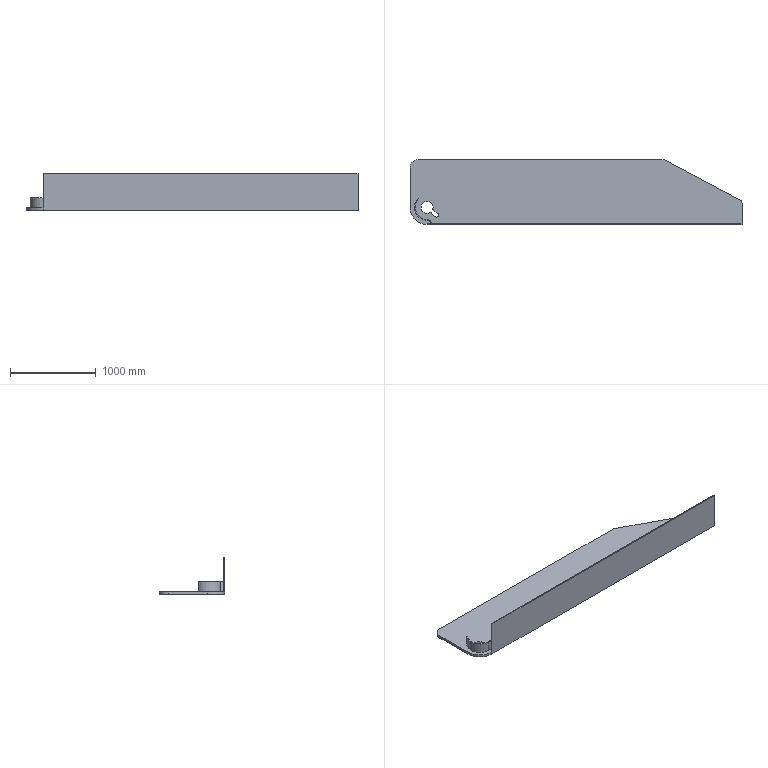Part | NX | features 顶梁侧护板右 2 | 1 solid | 26 faces | box 3880 x 760 x 430 mm | volume 99045232 mm3 | plane 14 | cylinder 12 | commonest cylinder face diameters 40 x2 50 x1 76 x1 96 x1 100 x1 140 x1
STEP:
#1=CARTESIAN_POINT('',(-1665.412,-207.572,-800.));
#2=VERTEX_POINT('',#1);
#3=CARTESIAN_POINT('',(-1673.791,-186.574,-800.));
#4=VERTEX_POINT('',#3);
#5=CARTESIAN_POINT('',(-1654.278,-190.958,-800.));
#6=DIRECTION('',(0.,0.,-1.));
#7=DIRECTION('',(1.,0.,0.));
#8=AXIS2_PLACEMENT_3D('',#5,#6,#7);
#9=CIRCLE('',#8,20.);
#10=EDGE_CURVE('',#2,#4,#9,.T.);
#11=ORIENTED_EDGE('',*,*,#10,.F.);
#12=CARTESIAN_POINT('',(-1619.198,-238.543,-800.));
#13=VERTEX_POINT('',#12);
#14=CARTESIAN_POINT('',(-1619.198,-238.543,-800.));
#15=DIRECTION('',(-0.8307,0.5567,0.));
#16=VECTOR('',#15,1000.);
#17=LINE('',#14,#16);
#18=EDGE_CURVE('',#13,#2,#17,.T.);
#19=ORIENTED_EDGE('',*,*,#18,.F.);
#20=CARTESIAN_POINT('',(-1650.504,-277.274,-800.));
#21=VERTEX_POINT('',#20);
#22=CARTESIAN_POINT('',(-1633.116,-259.311,-800.));
#23=DIRECTION('',(0.,0.,1.));
#24=DIRECTION('',(1.,0.,0.));
#25=AXIS2_PLACEMENT_3D('',#22,#23,#24);
#26=CIRCLE('',#25,25.);
#27=EDGE_CURVE('',#21,#13,#26,.T.);
#28=ORIENTED_EDGE('',*,*,#27,.F.);
#29=CARTESIAN_POINT('',(-1690.478,-238.583,-800.));
#30=VERTEX_POINT('',#29);
#31=CARTESIAN_POINT('',(-1690.478,-238.583,-800.));
#32=DIRECTION('',(0.7185,-0.6955,0.));
#33=VECTOR('',#32,1000.);
#34=LINE('',#31,#33);
#35=EDGE_CURVE('',#30,#21,#34,.T.);
#36=ORIENTED_EDGE('',*,*,#35,.F.);
#37=CARTESIAN_POINT('',(-1712.765,-234.793,-800.));
#38=VERTEX_POINT('',#37);
#39=CARTESIAN_POINT('',(-1704.387,-252.954,-800.));
#40=DIRECTION('',(0.,0.,-1.));
#41=DIRECTION('',(1.,0.,0.));
#42=AXIS2_PLACEMENT_3D('',#39,#40,#41);
#43=CIRCLE('',#42,20.);
#44=EDGE_CURVE('',#38,#30,#43,.T.);
#45=ORIENTED_EDGE('',*,*,#44,.F.);
#46=CARTESIAN_POINT('',(-1742.089,-171.231,-800.));
#47=DIRECTION('',(0.,0.,1.));
#48=DIRECTION('',(1.,0.,0.));
#49=AXIS2_PLACEMENT_3D('',#46,#47,#48);
#50=CIRCLE('',#49,70.);
#51=EDGE_CURVE('',#4,#38,#50,.T.);
#52=ORIENTED_EDGE('',*,*,#51,.F.);
#53=EDGE_LOOP('',(#11,#19,#28,#36,#45,#52));
#54=FACE_BOUND('',#53,.T.);
#55=CARTESIAN_POINT('',(-1742.089,-311.231,-800.));
#56=VERTEX_POINT('',#55);
#57=CARTESIAN_POINT('',(-1694.089,-359.231,-800.));
#58=VERTEX_POINT('',#57);
#59=CARTESIAN_POINT('',(-1742.089,-359.231,-800.));
#60=DIRECTION('',(0.,0.,-1.));
#61=DIRECTION('',(-1.,0.,0.));
#62=AXIS2_PLACEMENT_3D('',#59,#60,#61);
#63=CIRCLE('',#62,48.);
#64=EDGE_CURVE('',#56,#58,#63,.T.);
#65=ORIENTED_EDGE('',*,*,#64,.T.);
#66=CARTESIAN_POINT('',(1937.911,-359.231,-800.));
#67=VERTEX_POINT('',#66);
#68=CARTESIAN_POINT('',(1937.911,-359.231,-800.));
#69=DIRECTION('',(1.,0.,0.));
#70=VECTOR('',#69,1000.);
#71=LINE('',#68,#70);
#72=EDGE_CURVE('',#58,#67,#71,.T.);
#73=ORIENTED_EDGE('',*,*,#72,.T.);
#74=CARTESIAN_POINT('',(1937.911,-126.493,-800.));
#75=VERTEX_POINT('',#74);
#76=CARTESIAN_POINT('',(1937.911,-371.231,-800.));
#77=DIRECTION('',(0.,1.,0.));
#78=VECTOR('',#77,1000.);
#79=LINE('',#76,#78);
#80=EDGE_CURVE('',#67,#75,#79,.T.);
#81=ORIENTED_EDGE('',*,*,#80,.T.);
#82=CARTESIAN_POINT('',(1911.333,-82.318,-800.));
#83=VERTEX_POINT('',#82);
#84=CARTESIAN_POINT('',(1887.911,-126.493,-800.));
#85=DIRECTION('',(0.,0.,1.));
#86=DIRECTION('',(1.,0.,0.));
#87=AXIS2_PLACEMENT_3D('',#84,#85,#86);
#88=CIRCLE('',#87,50.);
#89=EDGE_CURVE('',#75,#83,#88,.T.);
#90=ORIENTED_EDGE('',*,*,#89,.T.);
#91=CARTESIAN_POINT('',(1040.435,379.448,-800.));
#92=VERTEX_POINT('',#91);
#93=CARTESIAN_POINT('',(1911.333,-82.318,-800.));
#94=DIRECTION('',(-0.8835,0.4684,0.));
#95=VECTOR('',#94,1000.);
#96=LINE('',#93,#95);
#97=EDGE_CURVE('',#83,#92,#96,.T.);
#98=ORIENTED_EDGE('',*,*,#97,.T.);
#99=CARTESIAN_POINT('',(1002.96,388.769,-800.));
#100=VERTEX_POINT('',#99);
#101=CARTESIAN_POINT('',(1002.96,308.769,-800.));
#102=DIRECTION('',(0.,0.,1.));
#103=DIRECTION('',(1.,0.,0.));
#104=AXIS2_PLACEMENT_3D('',#101,#102,#103);
#105=CIRCLE('',#104,80.);
#106=EDGE_CURVE('',#92,#100,#105,.T.);
#107=ORIENTED_EDGE('',*,*,#106,.T.);
#108=CARTESIAN_POINT('',(-1842.089,388.769,-800.));
#109=VERTEX_POINT('',#108);
#110=CARTESIAN_POINT('',(1002.96,388.769,-800.));
#111=DIRECTION('',(-1.,0.,0.));
#112=VECTOR('',#111,1000.);
#113=LINE('',#110,#112);
#114=EDGE_CURVE('',#100,#109,#113,.T.);
#115=ORIENTED_EDGE('',*,*,#114,.T.);
#116=CARTESIAN_POINT('',(-1942.089,288.769,-800.));
#117=VERTEX_POINT('',#116);
#118=CARTESIAN_POINT('',(-1842.089,288.769,-800.));
#119=DIRECTION('',(0.,0.,1.));
#120=DIRECTION('',(1.,0.,0.));
#121=AXIS2_PLACEMENT_3D('',#118,#119,#120);
#122=CIRCLE('',#121,100.);
#123=EDGE_CURVE('',#109,#117,#122,.T.);
#124=ORIENTED_EDGE('',*,*,#123,.T.);
#125=CARTESIAN_POINT('',(-1942.089,-171.231,-800.));
#126=VERTEX_POINT('',#125);
#127=CARTESIAN_POINT('',(-1942.089,288.769,-800.));
#128=DIRECTION('',(0.,-1.,0.));
#129=VECTOR('',#128,1000.);
#130=LINE('',#127,#129);
#131=EDGE_CURVE('',#117,#126,#130,.T.);
#132=ORIENTED_EDGE('',*,*,#131,.T.);
#133=CARTESIAN_POINT('',(-1742.089,-371.231,-800.));
#134=VERTEX_POINT('',#133);
#135=CARTESIAN_POINT('',(-1742.089,-171.231,-800.));
#136=DIRECTION('',(0.,0.,1.));
#137=DIRECTION('',(1.,0.,0.));
#138=AXIS2_PLACEMENT_3D('',#135,#136,#137);
#139=CIRCLE('',#138,200.);
#140=EDGE_CURVE('',#126,#134,#139,.T.);
#141=ORIENTED_EDGE('',*,*,#140,.T.);
#142=CARTESIAN_POINT('',(-1742.089,-359.231,-800.));
#143=VERTEX_POINT('',#142);
#144=CARTESIAN_POINT('',(-1742.089,-371.231,-800.));
#145=DIRECTION('',(0.,1.,0.));
#146=VECTOR('',#145,1000.);
#147=LINE('',#144,#146);
#148=EDGE_CURVE('',#134,#143,#147,.T.);
#149=ORIENTED_EDGE('',*,*,#148,.T.);
#150=CARTESIAN_POINT('',(-1704.089,-359.231,-800.));
#151=VERTEX_POINT('',#150);
#152=CARTESIAN_POINT('',(1937.911,-359.231,-800.));
#153=DIRECTION('',(1.,0.,0.));
#154=VECTOR('',#153,1000.);
#155=LINE('',#152,#154);
#156=EDGE_CURVE('',#143,#151,#155,.T.);
#157=ORIENTED_EDGE('',*,*,#156,.T.);
#158=CARTESIAN_POINT('',(-1742.089,-321.231,-800.));
#159=VERTEX_POINT('',#158);
#160=CARTESIAN_POINT('',(-1742.089,-359.231,-800.));
#161=DIRECTION('',(0.,0.,1.));
#162=DIRECTION('',(-1.,0.,0.));
#163=AXIS2_PLACEMENT_3D('',#160,#161,#162);
#164=CIRCLE('',#163,38.);
#165=EDGE_CURVE('',#151,#159,#164,.T.);
#166=ORIENTED_EDGE('',*,*,#165,.T.);
#167=CARTESIAN_POINT('',(-1848.155,-65.165,-800.));
#168=VERTEX_POINT('',#167);
#169=CARTESIAN_POINT('',(-1742.089,-171.231,-800.));
#170=DIRECTION('',(0.,0.,-1.));
#171=DIRECTION('',(-1.,0.,0.));
#172=AXIS2_PLACEMENT_3D('',#169,#170,#171);
#173=CIRCLE('',#172,150.);
#174=EDGE_CURVE('',#159,#168,#173,.T.);
#175=ORIENTED_EDGE('',*,*,#174,.T.);
#176=CARTESIAN_POINT('',(-1841.084,-72.237,-800.));
#177=VERTEX_POINT('',#176);
#178=CARTESIAN_POINT('',(-1841.084,-72.237,-800.));
#179=DIRECTION('',(0.7071,-0.7071,0.));
#180=VECTOR('',#179,1000.);
#181=LINE('',#178,#180);
#182=EDGE_CURVE('',#168,#177,#181,.T.);
#183=ORIENTED_EDGE('',*,*,#182,.T.);
#184=CARTESIAN_POINT('',(-1742.089,-171.231,-800.));
#185=DIRECTION('',(0.,0.,1.));
#186=DIRECTION('',(-1.,0.,0.));
#187=AXIS2_PLACEMENT_3D('',#184,#185,#186);
#188=CIRCLE('',#187,140.);
#189=EDGE_CURVE('',#177,#56,#188,.T.);
#190=ORIENTED_EDGE('',*,*,#189,.T.);
#191=EDGE_LOOP('',(#65,#73,#81,#90,#98,#107,#115,#124,#132,#141,#149,#157,#166,#175,#183,#190));
#192=FACE_BOUND('',#191,.T.);
#193=CARTESIAN_POINT('',(-1742.089,-171.231,-800.));
#194=DIRECTION('',(0.,0.,-1.));
#195=DIRECTION('',(1.,0.,0.));
#196=AXIS2_PLACEMENT_3D('',#193,#194,#195);
#197=PLANE('',#196);
#198=ADVANCED_FACE('',(#54,#192),#197,.F.);
#199=CARTESIAN_POINT('',(-1694.089,-359.231,-680.));
#200=VERTEX_POINT('',#199);
#201=CARTESIAN_POINT('',(-1694.089,-359.231,-680.));
#202=DIRECTION('',(0.,0.,-1.));
#203=VECTOR('',#202,1000.);
#204=LINE('',#201,#203);
#205=EDGE_CURVE('',#200,#58,#204,.T.);
#206=ORIENTED_EDGE('',*,*,#205,.F.);
#207=CARTESIAN_POINT('',(-1704.089,-359.231,-680.));
#208=VERTEX_POINT('',#207);
#209=CARTESIAN_POINT('',(-1694.089,-359.231,-680.));
#210=DIRECTION('',(-1.,0.,0.));
#211=VECTOR('',#210,1000.);
#212=LINE('',#209,#211);
#213=EDGE_CURVE('',#200,#208,#212,.T.);
#214=ORIENTED_EDGE('',*,*,#213,.T.);
#215=CARTESIAN_POINT('',(-1704.089,-359.231,-680.));
#216=DIRECTION('',(0.,0.,-1.));
#217=VECTOR('',#216,1000.);
#218=LINE('',#215,#217);
#219=EDGE_CURVE('',#208,#151,#218,.T.);
#220=ORIENTED_EDGE('',*,*,#219,.T.);
#221=ORIENTED_EDGE('',*,*,#156,.F.);
#222=CARTESIAN_POINT('',(-1742.089,-359.231,-400.));
#223=VERTEX_POINT('',#222);
#224=CARTESIAN_POINT('',(-1742.089,-359.231,-400.));
#225=DIRECTION('',(0.,0.,-1.));
#226=VECTOR('',#225,1000.);
#227=LINE('',#224,#226);
#228=EDGE_CURVE('',#223,#143,#227,.T.);
#229=ORIENTED_EDGE('',*,*,#228,.F.);
#230=CARTESIAN_POINT('',(1937.911,-359.231,-400.));
#231=VERTEX_POINT('',#230);
#232=CARTESIAN_POINT('',(1937.911,-359.231,-400.));
#233=DIRECTION('',(1.,0.,0.));
#234=VECTOR('',#233,1000.);
#235=LINE('',#232,#234);
#236=EDGE_CURVE('',#223,#231,#235,.T.);
#237=ORIENTED_EDGE('',*,*,#236,.T.);
#238=CARTESIAN_POINT('',(1937.911,-359.231,-400.));
#239=DIRECTION('',(0.,0.,-1.));
#240=VECTOR('',#239,1000.);
#241=LINE('',#238,#240);
#242=EDGE_CURVE('',#231,#67,#241,.T.);
#243=ORIENTED_EDGE('',*,*,#242,.T.);
#244=ORIENTED_EDGE('',*,*,#72,.F.);
#245=EDGE_LOOP('',(#206,#214,#220,#221,#229,#237,#243,#244));
#246=FACE_BOUND('',#245,.T.);
#247=CARTESIAN_POINT('',(1937.911,-359.231,-400.));
#248=DIRECTION('',(0.,-1.,0.));
#249=DIRECTION('',(0.,0.,1.));
#250=AXIS2_PLACEMENT_3D('',#247,#248,#249);
#251=PLANE('',#250);
#252=ADVANCED_FACE('',(#246),#251,.F.);
#253=CARTESIAN_POINT('',(-1942.089,-171.231,-830.));
#254=VERTEX_POINT('',#253);
#255=CARTESIAN_POINT('',(-1742.089,-371.231,-830.));
#256=VERTEX_POINT('',#255);
#257=CARTESIAN_POINT('',(-1742.089,-171.231,-830.));
#258=DIRECTION('',(0.,0.,1.));
#259=DIRECTION('',(1.,0.,0.));
#260=AXIS2_PLACEMENT_3D('',#257,#258,#259);
#261=CIRCLE('',#260,200.);
#262=EDGE_CURVE('',#254,#256,#261,.T.);
#263=ORIENTED_EDGE('',*,*,#262,.F.);
#264=CARTESIAN_POINT('',(-1942.089,288.769,-830.));
#265=VERTEX_POINT('',#264);
#266=CARTESIAN_POINT('',(-1942.089,288.769,-830.));
#267=DIRECTION('',(0.,-1.,0.));
#268=VECTOR('',#267,1000.);
#269=LINE('',#266,#268);
#270=EDGE_CURVE('',#265,#254,#269,.T.);
#271=ORIENTED_EDGE('',*,*,#270,.F.);
#272=CARTESIAN_POINT('',(-1842.089,388.769,-830.));
#273=VERTEX_POINT('',#272);
#274=CARTESIAN_POINT('',(-1842.089,288.769,-830.));
#275=DIRECTION('',(0.,0.,1.));
#276=DIRECTION('',(1.,0.,0.));
#277=AXIS2_PLACEMENT_3D('',#274,#275,#276);
#278=CIRCLE('',#277,100.);
#279=EDGE_CURVE('',#273,#265,#278,.T.);
#280=ORIENTED_EDGE('',*,*,#279,.F.);
#281=CARTESIAN_POINT('',(1002.96,388.769,-830.));
#282=VERTEX_POINT('',#281);
#283=CARTESIAN_POINT('',(1002.96,388.769,-830.));
#284=DIRECTION('',(-1.,0.,0.));
#285=VECTOR('',#284,1000.);
#286=LINE('',#283,#285);
#287=EDGE_CURVE('',#282,#273,#286,.T.);
#288=ORIENTED_EDGE('',*,*,#287,.F.);
#289=CARTESIAN_POINT('',(1040.435,379.448,-830.));
#290=VERTEX_POINT('',#289);
#291=CARTESIAN_POINT('',(1002.96,308.769,-830.));
#292=DIRECTION('',(0.,0.,1.));
#293=DIRECTION('',(1.,0.,0.));
#294=AXIS2_PLACEMENT_3D('',#291,#292,#293);
#295=CIRCLE('',#294,80.);
#296=EDGE_CURVE('',#290,#282,#295,.T.);
#297=ORIENTED_EDGE('',*,*,#296,.F.);
#298=CARTESIAN_POINT('',(1911.333,-82.318,-830.));
#299=VERTEX_POINT('',#298);
#300=CARTESIAN_POINT('',(1911.333,-82.318,-830.));
#301=DIRECTION('',(-0.8835,0.4684,0.));
#302=VECTOR('',#301,1000.);
#303=LINE('',#300,#302);
#304=EDGE_CURVE('',#299,#290,#303,.T.);
#305=ORIENTED_EDGE('',*,*,#304,.F.);
#306=CARTESIAN_POINT('',(1937.911,-126.493,-830.));
#307=VERTEX_POINT('',#306);
#308=CARTESIAN_POINT('',(1887.911,-126.493,-830.));
#309=DIRECTION('',(0.,0.,1.));
#310=DIRECTION('',(1.,0.,0.));
#311=AXIS2_PLACEMENT_3D('',#308,#309,#310);
#312=CIRCLE('',#311,50.);
#313=EDGE_CURVE('',#307,#299,#312,.T.);
#314=ORIENTED_EDGE('',*,*,#313,.F.);
#315=CARTESIAN_POINT('',(1937.911,-371.231,-830.));
#316=VERTEX_POINT('',#315);
#317=CARTESIAN_POINT('',(1937.911,-371.231,-830.));
#318=DIRECTION('',(0.,1.,0.));
#319=VECTOR('',#318,1000.);
#320=LINE('',#317,#319);
#321=EDGE_CURVE('',#316,#307,#320,.T.);
#322=ORIENTED_EDGE('',*,*,#321,.F.);
#323=CARTESIAN_POINT('',(-1742.089,-371.231,-830.));
#324=DIRECTION('',(1.,0.,0.));
#325=VECTOR('',#324,1000.);
#326=LINE('',#323,#325);
#327=EDGE_CURVE('',#256,#316,#326,.T.);
#328=ORIENTED_EDGE('',*,*,#327,.F.);
#329=EDGE_LOOP('',(#263,#271,#280,#288,#297,#305,#314,#322,#328));
#330=FACE_BOUND('',#329,.T.);
#331=CARTESIAN_POINT('',(-1673.791,-186.574,-830.));
#332=VERTEX_POINT('',#331);
#333=CARTESIAN_POINT('',(-1712.765,-234.793,-830.));
#334=VERTEX_POINT('',#333);
#335=CARTESIAN_POINT('',(-1742.089,-171.231,-830.));
#336=DIRECTION('',(0.,0.,1.));
#337=DIRECTION('',(1.,0.,0.));
#338=AXIS2_PLACEMENT_3D('',#335,#336,#337);
#339=CIRCLE('',#338,70.);
#340=EDGE_CURVE('',#332,#334,#339,.T.);
#341=ORIENTED_EDGE('',*,*,#340,.T.);
#342=CARTESIAN_POINT('',(-1690.478,-238.583,-830.));
#343=VERTEX_POINT('',#342);
#344=CARTESIAN_POINT('',(-1704.387,-252.954,-830.));
#345=DIRECTION('',(0.,0.,-1.));
#346=DIRECTION('',(1.,0.,0.));
#347=AXIS2_PLACEMENT_3D('',#344,#345,#346);
#348=CIRCLE('',#347,20.);
#349=EDGE_CURVE('',#334,#343,#348,.T.);
#350=ORIENTED_EDGE('',*,*,#349,.T.);
#351=CARTESIAN_POINT('',(-1650.504,-277.274,-830.));
#352=VERTEX_POINT('',#351);
#353=CARTESIAN_POINT('',(-1690.478,-238.583,-830.));
#354=DIRECTION('',(0.7185,-0.6955,0.));
#355=VECTOR('',#354,1000.);
#356=LINE('',#353,#355);
#357=EDGE_CURVE('',#343,#352,#356,.T.);
#358=ORIENTED_EDGE('',*,*,#357,.T.);
#359=CARTESIAN_POINT('',(-1619.198,-238.543,-830.));
#360=VERTEX_POINT('',#359);
#361=CARTESIAN_POINT('',(-1633.116,-259.311,-830.));
#362=DIRECTION('',(0.,0.,1.));
#363=DIRECTION('',(1.,0.,0.));
#364=AXIS2_PLACEMENT_3D('',#361,#362,#363);
#365=CIRCLE('',#364,25.);
#366=EDGE_CURVE('',#352,#360,#365,.T.);
#367=ORIENTED_EDGE('',*,*,#366,.T.);
#368=CARTESIAN_POINT('',(-1665.412,-207.572,-830.));
#369=VERTEX_POINT('',#368);
#370=CARTESIAN_POINT('',(-1619.198,-238.543,-830.));
#371=DIRECTION('',(-0.8307,0.5567,0.));
#372=VECTOR('',#371,1000.);
#373=LINE('',#370,#372);
#374=EDGE_CURVE('',#360,#369,#373,.T.);
#375=ORIENTED_EDGE('',*,*,#374,.T.);
#376=CARTESIAN_POINT('',(-1654.278,-190.958,-830.));
#377=DIRECTION('',(0.,0.,-1.));
#378=DIRECTION('',(1.,0.,0.));
#379=AXIS2_PLACEMENT_3D('',#376,#377,#378);
#380=CIRCLE('',#379,20.);
#381=EDGE_CURVE('',#369,#332,#380,.T.);
#382=ORIENTED_EDGE('',*,*,#381,.T.);
#383=EDGE_LOOP('',(#341,#350,#358,#367,#375,#382));
#384=FACE_BOUND('',#383,.T.);
#385=CARTESIAN_POINT('',(-1742.089,-171.231,-830.));
#386=DIRECTION('',(0.,0.,-1.));
#387=DIRECTION('',(1.,0.,0.));
#388=AXIS2_PLACEMENT_3D('',#385,#386,#387);
#389=PLANE('',#388);
#390=ADVANCED_FACE('',(#330,#384),#389,.T.);
#391=ORIENTED_EDGE('',*,*,#140,.F.);
#392=CARTESIAN_POINT('',(-1942.089,-171.231,-830.));
#393=DIRECTION('',(0.,0.,1.));
#394=VECTOR('',#393,1000.);
#395=LINE('',#392,#394);
#396=EDGE_CURVE('',#254,#126,#395,.T.);
#397=ORIENTED_EDGE('',*,*,#396,.F.);
#398=ORIENTED_EDGE('',*,*,#262,.T.);
#399=CARTESIAN_POINT('',(-1742.089,-371.231,-830.));
#400=DIRECTION('',(0.,0.,1.));
#401=VECTOR('',#400,1000.);
#402=LINE('',#399,#401);
#403=EDGE_CURVE('',#256,#134,#402,.T.);
#404=ORIENTED_EDGE('',*,*,#403,.T.);
#405=EDGE_LOOP('',(#391,#397,#398,#404));
#406=FACE_BOUND('',#405,.T.);
#407=CARTESIAN_POINT('',(-1742.089,-171.231,-830.));
#408=DIRECTION('',(0.,0.,1.));
#409=DIRECTION('',(-1.,0.,0.));
#410=AXIS2_PLACEMENT_3D('',#407,#408,#409);
#411=CYLINDRICAL_SURFACE('',#410,200.);
#412=ADVANCED_FACE('',(#406),#411,.T.);
#413=ORIENTED_EDGE('',*,*,#403,.F.);
#414=ORIENTED_EDGE('',*,*,#327,.T.);
#415=CARTESIAN_POINT('',(1937.911,-371.231,-400.));
#416=VERTEX_POINT('',#415);
#417=CARTESIAN_POINT('',(1937.911,-371.231,-830.));
#418=DIRECTION('',(0.,0.,1.));
#419=VECTOR('',#418,1000.);
#420=LINE('',#417,#419);
#421=EDGE_CURVE('',#316,#416,#420,.T.);
#422=ORIENTED_EDGE('',*,*,#421,.T.);
#423=CARTESIAN_POINT('',(-1742.089,-371.231,-400.));
#424=VERTEX_POINT('',#423);
#425=CARTESIAN_POINT('',(1937.911,-371.231,-400.));
#426=DIRECTION('',(-1.,0.,0.));
#427=VECTOR('',#426,1000.);
#428=LINE('',#425,#427);
#429=EDGE_CURVE('',#416,#424,#428,.T.);
#430=ORIENTED_EDGE('',*,*,#429,.T.);
#431=CARTESIAN_POINT('',(-1742.089,-371.231,-400.));
#432=DIRECTION('',(0.,0.,-1.));
#433=VECTOR('',#432,1000.);
#434=LINE('',#431,#433);
#435=EDGE_CURVE('',#424,#134,#434,.T.);
#436=ORIENTED_EDGE('',*,*,#435,.T.);
#437=EDGE_LOOP('',(#413,#414,#422,#430,#436));
#438=FACE_BOUND('',#437,.T.);
#439=CARTESIAN_POINT('',(-1742.089,-371.231,-830.));
#440=DIRECTION('',(0.,1.,0.));
#441=DIRECTION('',(0.,0.,-1.));
#442=AXIS2_PLACEMENT_3D('',#439,#440,#441);
#443=PLANE('',#442);
#444=ADVANCED_FACE('',(#438),#443,.F.);
#445=ORIENTED_EDGE('',*,*,#421,.F.);
#446=ORIENTED_EDGE('',*,*,#321,.T.);
#447=CARTESIAN_POINT('',(1937.911,-126.493,-830.));
#448=DIRECTION('',(0.,0.,1.));
#449=VECTOR('',#448,1000.);
#450=LINE('',#447,#449);
#451=EDGE_CURVE('',#307,#75,#450,.T.);
#452=ORIENTED_EDGE('',*,*,#451,.T.);
#453=ORIENTED_EDGE('',*,*,#80,.F.);
#454=ORIENTED_EDGE('',*,*,#242,.F.);
#455=CARTESIAN_POINT('',(1937.911,-371.231,-400.));
#456=DIRECTION('',(0.,-1.,0.));
#457=VECTOR('',#456,1000.);
#458=LINE('',#455,#457);
#459=EDGE_CURVE('',#231,#416,#458,.T.);
#460=ORIENTED_EDGE('',*,*,#459,.T.);
#461=EDGE_LOOP('',(#445,#446,#452,#453,#454,#460));
#462=FACE_BOUND('',#461,.T.);
#463=CARTESIAN_POINT('',(1937.911,-371.231,-830.));
#464=DIRECTION('',(-1.,0.,0.));
#465=DIRECTION('',(0.,0.,-1.));
#466=AXIS2_PLACEMENT_3D('',#463,#464,#465);
#467=PLANE('',#466);
#468=ADVANCED_FACE('',(#462),#467,.F.);
#469=ORIENTED_EDGE('',*,*,#89,.F.);
#470=ORIENTED_EDGE('',*,*,#451,.F.);
#471=ORIENTED_EDGE('',*,*,#313,.T.);
#472=CARTESIAN_POINT('',(1911.333,-82.318,-830.));
#473=DIRECTION('',(0.,0.,1.));
#474=VECTOR('',#473,1000.);
#475=LINE('',#472,#474);
#476=EDGE_CURVE('',#299,#83,#475,.T.);
#477=ORIENTED_EDGE('',*,*,#476,.T.);
#478=EDGE_LOOP('',(#469,#470,#471,#477));
#479=FACE_BOUND('',#478,.T.);
#480=CARTESIAN_POINT('',(1887.911,-126.493,-830.));
#481=DIRECTION('',(0.,0.,1.));
#482=DIRECTION('',(-1.,0.,0.));
#483=AXIS2_PLACEMENT_3D('',#480,#481,#482);
#484=CYLINDRICAL_SURFACE('',#483,50.);
#485=ADVANCED_FACE('',(#479),#484,.T.);
#486=ORIENTED_EDGE('',*,*,#97,.F.);
#487=ORIENTED_EDGE('',*,*,#476,.F.);
#488=ORIENTED_EDGE('',*,*,#304,.T.);
#489=CARTESIAN_POINT('',(1040.435,379.448,-830.));
#490=DIRECTION('',(0.,0.,1.));
#491=VECTOR('',#490,1000.);
#492=LINE('',#489,#491);
#493=EDGE_CURVE('',#290,#92,#492,.T.);
#494=ORIENTED_EDGE('',*,*,#493,.T.);
#495=EDGE_LOOP('',(#486,#487,#488,#494));
#496=FACE_BOUND('',#495,.T.);
#497=CARTESIAN_POINT('',(1911.333,-82.318,-830.));
#498=DIRECTION('',(-0.4684,-0.8835,0.));
#499=DIRECTION('',(0.8835,-0.4684,0.));
#500=AXIS2_PLACEMENT_3D('',#497,#498,#499);
#501=PLANE('',#500);
#502=ADVANCED_FACE('',(#496),#501,.F.);
#503=ORIENTED_EDGE('',*,*,#106,.F.);
#504=ORIENTED_EDGE('',*,*,#493,.F.);
#505=ORIENTED_EDGE('',*,*,#296,.T.);
#506=CARTESIAN_POINT('',(1002.96,388.769,-830.));
#507=DIRECTION('',(0.,0.,1.));
#508=VECTOR('',#507,1000.);
#509=LINE('',#506,#508);
#510=EDGE_CURVE('',#282,#100,#509,.T.);
#511=ORIENTED_EDGE('',*,*,#510,.T.);
#512=EDGE_LOOP('',(#503,#504,#505,#511));
#513=FACE_BOUND('',#512,.T.);
#514=CARTESIAN_POINT('',(1002.96,308.769,-830.));
#515=DIRECTION('',(0.,0.,1.));
#516=DIRECTION('',(-1.,0.,0.));
#517=AXIS2_PLACEMENT_3D('',#514,#515,#516);
#518=CYLINDRICAL_SURFACE('',#517,80.);
#519=ADVANCED_FACE('',(#513),#518,.T.);
#520=ORIENTED_EDGE('',*,*,#114,.F.);
#521=ORIENTED_EDGE('',*,*,#510,.F.);
#522=ORIENTED_EDGE('',*,*,#287,.T.);
#523=CARTESIAN_POINT('',(-1842.089,388.769,-830.));
#524=DIRECTION('',(0.,0.,1.));
#525=VECTOR('',#524,1000.);
#526=LINE('',#523,#525);
#527=EDGE_CURVE('',#273,#109,#526,.T.);
#528=ORIENTED_EDGE('',*,*,#527,.T.);
#529=EDGE_LOOP('',(#520,#521,#522,#528));
#530=FACE_BOUND('',#529,.T.);
#531=CARTESIAN_POINT('',(1002.96,388.769,-830.));
#532=DIRECTION('',(0.,-1.,0.));
#533=DIRECTION('',(0.,0.,1.));
#534=AXIS2_PLACEMENT_3D('',#531,#532,#533);
#535=PLANE('',#534);
#536=ADVANCED_FACE('',(#530),#535,.F.);
#537=ORIENTED_EDGE('',*,*,#123,.F.);
#538=ORIENTED_EDGE('',*,*,#527,.F.);
#539=ORIENTED_EDGE('',*,*,#279,.T.);
#540=CARTESIAN_POINT('',(-1942.089,288.769,-830.));
#541=DIRECTION('',(0.,0.,1.));
#542=VECTOR('',#541,1000.);
#543=LINE('',#540,#542);
#544=EDGE_CURVE('',#265,#117,#543,.T.);
#545=ORIENTED_EDGE('',*,*,#544,.T.);
#546=EDGE_LOOP('',(#537,#538,#539,#545));
#547=FACE_BOUND('',#546,.T.);
#548=CARTESIAN_POINT('',(-1842.089,288.769,-830.));
#549=DIRECTION('',(0.,0.,1.));
#550=DIRECTION('',(-1.,0.,0.));
#551=AXIS2_PLACEMENT_3D('',#548,#549,#550);
#552=CYLINDRICAL_SURFACE('',#551,100.);
#553=ADVANCED_FACE('',(#547),#552,.T.);
#554=ORIENTED_EDGE('',*,*,#131,.F.);
#555=ORIENTED_EDGE('',*,*,#544,.F.);
#556=ORIENTED_EDGE('',*,*,#270,.T.);
#557=ORIENTED_EDGE('',*,*,#396,.T.);
#558=EDGE_LOOP('',(#554,#555,#556,#557));
#559=FACE_BOUND('',#558,.T.);
#560=CARTESIAN_POINT('',(-1942.089,288.769,-830.));
#561=DIRECTION('',(1.,0.,0.));
#562=DIRECTION('',(0.,0.,1.));
#563=AXIS2_PLACEMENT_3D('',#560,#561,#562);
#564=PLANE('',#563);
#565=ADVANCED_FACE('',(#559),#564,.F.);
#566=ORIENTED_EDGE('',*,*,#10,.T.);
#567=CARTESIAN_POINT('',(-1673.791,-186.574,-830.));
#568=DIRECTION('',(0.,0.,1.));
#569=VECTOR('',#568,1000.);
#570=LINE('',#567,#569);
#571=EDGE_CURVE('',#332,#4,#570,.T.);
#572=ORIENTED_EDGE('',*,*,#571,.F.);
#573=ORIENTED_EDGE('',*,*,#381,.F.);
#574=CARTESIAN_POINT('',(-1665.412,-207.572,-830.));
#575=DIRECTION('',(0.,0.,1.));
#576=VECTOR('',#575,1000.);
#577=LINE('',#574,#576);
#578=EDGE_CURVE('',#369,#2,#577,.T.);
#579=ORIENTED_EDGE('',*,*,#578,.T.);
#580=EDGE_LOOP('',(#566,#572,#573,#579));
#581=FACE_BOUND('',#580,.T.);
#582=CARTESIAN_POINT('',(-1654.278,-190.958,-830.));
#583=DIRECTION('',(0.,0.,1.));
#584=DIRECTION('',(-1.,0.,0.));
#585=AXIS2_PLACEMENT_3D('',#582,#583,#584);
#586=CYLINDRICAL_SURFACE('',#585,20.);
#587=ADVANCED_FACE('',(#581),#586,.T.);
#588=ORIENTED_EDGE('',*,*,#51,.T.);
#589=CARTESIAN_POINT('',(-1712.765,-234.793,-830.));
#590=DIRECTION('',(0.,0.,1.));
#591=VECTOR('',#590,1000.);
#592=LINE('',#589,#591);
#593=EDGE_CURVE('',#334,#38,#592,.T.);
#594=ORIENTED_EDGE('',*,*,#593,.F.);
#595=ORIENTED_EDGE('',*,*,#340,.F.);
#596=ORIENTED_EDGE('',*,*,#571,.T.);
#597=EDGE_LOOP('',(#588,#594,#595,#596));
#598=FACE_BOUND('',#597,.T.);
#599=CARTESIAN_POINT('',(-1742.089,-171.231,-830.));
#600=DIRECTION('',(0.,0.,1.));
#601=DIRECTION('',(-1.,0.,0.));
#602=AXIS2_PLACEMENT_3D('',#599,#600,#601);
#603=CYLINDRICAL_SURFACE('',#602,70.);
#604=ADVANCED_FACE('',(#598),#603,.F.);
#605=ORIENTED_EDGE('',*,*,#44,.T.);
#606=CARTESIAN_POINT('',(-1690.478,-238.583,-830.));
#607=DIRECTION('',(0.,0.,1.));
#608=VECTOR('',#607,1000.);
#609=LINE('',#606,#608);
#610=EDGE_CURVE('',#343,#30,#609,.T.);
#611=ORIENTED_EDGE('',*,*,#610,.F.);
#612=ORIENTED_EDGE('',*,*,#349,.F.);
#613=ORIENTED_EDGE('',*,*,#593,.T.);
#614=EDGE_LOOP('',(#605,#611,#612,#613));
#615=FACE_BOUND('',#614,.T.);
#616=CARTESIAN_POINT('',(-1704.387,-252.954,-830.));
#617=DIRECTION('',(0.,0.,1.));
#618=DIRECTION('',(-1.,0.,0.));
#619=AXIS2_PLACEMENT_3D('',#616,#617,#618);
#620=CYLINDRICAL_SURFACE('',#619,20.);
#621=ADVANCED_FACE('',(#615),#620,.T.);
#622=ORIENTED_EDGE('',*,*,#35,.T.);
#623=CARTESIAN_POINT('',(-1650.504,-277.274,-830.));
#624=DIRECTION('',(0.,0.,1.));
#625=VECTOR('',#624,1000.);
#626=LINE('',#623,#625);
#627=EDGE_CURVE('',#352,#21,#626,.T.);
#628=ORIENTED_EDGE('',*,*,#627,.F.);
#629=ORIENTED_EDGE('',*,*,#357,.F.);
#630=ORIENTED_EDGE('',*,*,#610,.T.);
#631=EDGE_LOOP('',(#622,#628,#629,#630));
#632=FACE_BOUND('',#631,.T.);
#633=CARTESIAN_POINT('',(-1690.478,-238.583,-830.));
#634=DIRECTION('',(0.6955,0.7185,0.));
#635=DIRECTION('',(-0.7185,0.6955,0.));
#636=AXIS2_PLACEMENT_3D('',#633,#634,#635);
#637=PLANE('',#636);
#638=ADVANCED_FACE('',(#632),#637,.T.);
#639=ORIENTED_EDGE('',*,*,#27,.T.);
#640=CARTESIAN_POINT('',(-1619.198,-238.543,-830.));
#641=DIRECTION('',(0.,0.,1.));
#642=VECTOR('',#641,1000.);
#643=LINE('',#640,#642);
#644=EDGE_CURVE('',#360,#13,#643,.T.);
#645=ORIENTED_EDGE('',*,*,#644,.F.);
#646=ORIENTED_EDGE('',*,*,#366,.F.);
#647=ORIENTED_EDGE('',*,*,#627,.T.);
#648=EDGE_LOOP('',(#639,#645,#646,#647));
#649=FACE_BOUND('',#648,.T.);
#650=CARTESIAN_POINT('',(-1633.116,-259.311,-830.));
#651=DIRECTION('',(0.,0.,1.));
#652=DIRECTION('',(-1.,0.,0.));
#653=AXIS2_PLACEMENT_3D('',#650,#651,#652);
#654=CYLINDRICAL_SURFACE('',#653,25.);
#655=ADVANCED_FACE('',(#649),#654,.F.);
#656=ORIENTED_EDGE('',*,*,#18,.T.);
#657=ORIENTED_EDGE('',*,*,#578,.F.);
#658=ORIENTED_EDGE('',*,*,#374,.F.);
#659=ORIENTED_EDGE('',*,*,#644,.T.);
#660=EDGE_LOOP('',(#656,#657,#658,#659));
#661=FACE_BOUND('',#660,.T.);
#662=CARTESIAN_POINT('',(-1619.198,-238.543,-830.));
#663=DIRECTION('',(-0.5567,-0.8307,0.));
#664=DIRECTION('',(0.8307,-0.5567,0.));
#665=AXIS2_PLACEMENT_3D('',#662,#663,#664);
#666=PLANE('',#665);
#667=ADVANCED_FACE('',(#661),#666,.T.);
#668=ORIENTED_EDGE('',*,*,#148,.F.);
#669=ORIENTED_EDGE('',*,*,#435,.F.);
#670=CARTESIAN_POINT('',(-1742.089,-371.231,-400.));
#671=DIRECTION('',(0.,1.,0.));
#672=VECTOR('',#671,1000.);
#673=LINE('',#670,#672);
#674=EDGE_CURVE('',#424,#223,#673,.T.);
#675=ORIENTED_EDGE('',*,*,#674,.T.);
#676=ORIENTED_EDGE('',*,*,#228,.T.);
#677=EDGE_LOOP('',(#668,#669,#675,#676));
#678=FACE_BOUND('',#677,.T.);
#679=CARTESIAN_POINT('',(-1742.089,-371.231,-400.));
#680=DIRECTION('',(1.,0.,0.));
#681=DIRECTION('',(0.,0.,1.));
#682=AXIS2_PLACEMENT_3D('',#679,#680,#681);
#683=PLANE('',#682);
#684=ADVANCED_FACE('',(#678),#683,.F.);
#685=ORIENTED_EDGE('',*,*,#459,.F.);
#686=ORIENTED_EDGE('',*,*,#236,.F.);
#687=ORIENTED_EDGE('',*,*,#674,.F.);
#688=ORIENTED_EDGE('',*,*,#429,.F.);
#689=EDGE_LOOP('',(#685,#686,#687,#688));
#690=FACE_BOUND('',#689,.T.);
#691=CARTESIAN_POINT('',(1937.911,-359.231,-400.));
#692=DIRECTION('',(0.,0.,-1.));
#693=DIRECTION('',(1.,0.,0.));
#694=AXIS2_PLACEMENT_3D('',#691,#692,#693);
#695=PLANE('',#694);
#696=ADVANCED_FACE('',(#690),#695,.F.);
#697=ORIENTED_EDGE('',*,*,#189,.F.);
#698=CARTESIAN_POINT('',(-1841.084,-72.237,-680.));
#699=VERTEX_POINT('',#698);
#700=CARTESIAN_POINT('',(-1841.084,-72.237,-680.));
#701=DIRECTION('',(0.,0.,-1.));
#702=VECTOR('',#701,1000.);
#703=LINE('',#700,#702);
#704=EDGE_CURVE('',#699,#177,#703,.T.);
#705=ORIENTED_EDGE('',*,*,#704,.F.);
#706=CARTESIAN_POINT('',(-1742.089,-311.231,-680.));
#707=VERTEX_POINT('',#706);
#708=CARTESIAN_POINT('',(-1742.089,-171.231,-680.));
#709=DIRECTION('',(0.,0.,1.));
#710=DIRECTION('',(-1.,0.,0.));
#711=AXIS2_PLACEMENT_3D('',#708,#709,#710);
#712=CIRCLE('',#711,140.);
#713=EDGE_CURVE('',#699,#707,#712,.T.);
#714=ORIENTED_EDGE('',*,*,#713,.T.);
#715=CARTESIAN_POINT('',(-1742.089,-311.231,-680.));
#716=DIRECTION('',(0.,0.,-1.));
#717=VECTOR('',#716,1000.);
#718=LINE('',#715,#717);
#719=EDGE_CURVE('',#707,#56,#718,.T.);
#720=ORIENTED_EDGE('',*,*,#719,.T.);
#721=EDGE_LOOP('',(#697,#705,#714,#720));
#722=FACE_BOUND('',#721,.T.);
#723=CARTESIAN_POINT('',(-1742.089,-171.231,-680.));
#724=DIRECTION('',(0.,0.,-1.));
#725=DIRECTION('',(1.,0.,0.));
#726=AXIS2_PLACEMENT_3D('',#723,#724,#725);
#727=CYLINDRICAL_SURFACE('',#726,140.);
#728=ADVANCED_FACE('',(#722),#727,.F.);
#729=ORIENTED_EDGE('',*,*,#64,.F.);
#730=ORIENTED_EDGE('',*,*,#719,.F.);
#731=CARTESIAN_POINT('',(-1742.089,-359.231,-680.));
#732=DIRECTION('',(0.,0.,-1.));
#733=DIRECTION('',(-1.,0.,0.));
#734=AXIS2_PLACEMENT_3D('',#731,#732,#733);
#735=CIRCLE('',#734,48.);
#736=EDGE_CURVE('',#707,#200,#735,.T.);
#737=ORIENTED_EDGE('',*,*,#736,.T.);
#738=ORIENTED_EDGE('',*,*,#205,.T.);
#739=EDGE_LOOP('',(#729,#730,#737,#738));
#740=FACE_BOUND('',#739,.T.);
#741=CARTESIAN_POINT('',(-1742.089,-359.231,-680.));
#742=DIRECTION('',(0.,0.,-1.));
#743=DIRECTION('',(1.,0.,0.));
#744=AXIS2_PLACEMENT_3D('',#741,#742,#743);
#745=CYLINDRICAL_SURFACE('',#744,48.);
#746=ADVANCED_FACE('',(#740),#745,.T.);
#747=ORIENTED_EDGE('',*,*,#165,.F.);
#748=ORIENTED_EDGE('',*,*,#219,.F.);
#749=CARTESIAN_POINT('',(-1742.089,-321.231,-680.));
#750=VERTEX_POINT('',#749);
#751=CARTESIAN_POINT('',(-1742.089,-359.231,-680.));
#752=DIRECTION('',(0.,0.,1.));
#753=DIRECTION('',(-1.,0.,0.));
#754=AXIS2_PLACEMENT_3D('',#751,#752,#753);
#755=CIRCLE('',#754,38.);
#756=EDGE_CURVE('',#208,#750,#755,.T.);
#757=ORIENTED_EDGE('',*,*,#756,.T.);
#758=CARTESIAN_POINT('',(-1742.089,-321.231,-680.));
#759=DIRECTION('',(0.,0.,-1.));
#760=VECTOR('',#759,1000.);
#761=LINE('',#758,#760);
#762=EDGE_CURVE('',#750,#159,#761,.T.);
#763=ORIENTED_EDGE('',*,*,#762,.T.);
#764=EDGE_LOOP('',(#747,#748,#757,#763));
#765=FACE_BOUND('',#764,.T.);
#766=CARTESIAN_POINT('',(-1742.089,-359.231,-680.));
#767=DIRECTION('',(0.,0.,-1.));
#768=DIRECTION('',(1.,0.,0.));
#769=AXIS2_PLACEMENT_3D('',#766,#767,#768);
#770=CYLINDRICAL_SURFACE('',#769,38.);
#771=ADVANCED_FACE('',(#765),#770,.F.);
#772=ORIENTED_EDGE('',*,*,#174,.F.);
#773=ORIENTED_EDGE('',*,*,#762,.F.);
#774=CARTESIAN_POINT('',(-1848.155,-65.165,-680.));
#775=VERTEX_POINT('',#774);
#776=CARTESIAN_POINT('',(-1742.089,-171.231,-680.));
#777=DIRECTION('',(0.,0.,-1.));
#778=DIRECTION('',(-1.,0.,0.));
#779=AXIS2_PLACEMENT_3D('',#776,#777,#778);
#780=CIRCLE('',#779,150.);
#781=EDGE_CURVE('',#750,#775,#780,.T.);
#782=ORIENTED_EDGE('',*,*,#781,.T.);
#783=CARTESIAN_POINT('',(-1848.155,-65.165,-680.));
#784=DIRECTION('',(0.,0.,-1.));
#785=VECTOR('',#784,1000.);
#786=LINE('',#783,#785);
#787=EDGE_CURVE('',#775,#168,#786,.T.);
#788=ORIENTED_EDGE('',*,*,#787,.T.);
#789=EDGE_LOOP('',(#772,#773,#782,#788));
#790=FACE_BOUND('',#789,.T.);
#791=CARTESIAN_POINT('',(-1742.089,-171.231,-680.));
#792=DIRECTION('',(0.,0.,-1.));
#793=DIRECTION('',(1.,0.,0.));
#794=AXIS2_PLACEMENT_3D('',#791,#792,#793);
#795=CYLINDRICAL_SURFACE('',#794,150.);
#796=ADVANCED_FACE('',(#790),#795,.T.);
#797=ORIENTED_EDGE('',*,*,#182,.F.);
#798=ORIENTED_EDGE('',*,*,#787,.F.);
#799=CARTESIAN_POINT('',(-1841.084,-72.237,-680.));
#800=DIRECTION('',(0.7071,-0.7071,0.));
#801=VECTOR('',#800,1000.);
#802=LINE('',#799,#801);
#803=EDGE_CURVE('',#775,#699,#802,.T.);
#804=ORIENTED_EDGE('',*,*,#803,.T.);
#805=ORIENTED_EDGE('',*,*,#704,.T.);
#806=EDGE_LOOP('',(#797,#798,#804,#805));
#807=FACE_BOUND('',#806,.T.);
#808=CARTESIAN_POINT('',(-1841.084,-72.237,-680.));
#809=DIRECTION('',(-0.7071,-0.7071,0.));
#810=DIRECTION('',(0.7071,-0.7071,0.));
#811=AXIS2_PLACEMENT_3D('',#808,#809,#810);
#812=PLANE('',#811);
#813=ADVANCED_FACE('',(#807),#812,.F.);
#814=ORIENTED_EDGE('',*,*,#713,.F.);
#815=ORIENTED_EDGE('',*,*,#803,.F.);
#816=ORIENTED_EDGE('',*,*,#781,.F.);
#817=ORIENTED_EDGE('',*,*,#756,.F.);
#818=ORIENTED_EDGE('',*,*,#213,.F.);
#819=ORIENTED_EDGE('',*,*,#736,.F.);
#820=EDGE_LOOP('',(#814,#815,#816,#817,#818,#819));
#821=FACE_BOUND('',#820,.T.);
#822=CARTESIAN_POINT('',(-1742.089,-171.231,-680.));
#823=DIRECTION('',(0.,0.,1.));
#824=DIRECTION('',(-1.,0.,0.));
#825=AXIS2_PLACEMENT_3D('',#822,#823,#824);
#826=PLANE('',#825);
#827=ADVANCED_FACE('',(#821),#826,.T.);
#828=CLOSED_SHELL('',(#198,#252,#390,#412,#444,#468,#485,#502,#519,#536,#553,#565,#587,#604,#621,#638,#655,#667,#684,#696,#728,#746,#771,#796,#813,#827));
#829=MANIFOLD_SOLID_BREP('',#828);
#830=(LENGTH_UNIT()NAMED_UNIT(*)SI_UNIT(.MILLI.,.METRE.));
#831=UNCERTAINTY_MEASURE_WITH_UNIT(LENGTH_MEASURE(0.00001),#830,'','');
#832=(NAMED_UNIT(*)PLANE_ANGLE_UNIT()SI_UNIT($,.RADIAN.));
#833=(NAMED_UNIT(*)SI_UNIT($,.STERADIAN.)SOLID_ANGLE_UNIT());
#834=(GEOMETRIC_REPRESENTATION_CONTEXT(3)GLOBAL_UNCERTAINTY_ASSIGNED_CONTEXT((#831))GLOBAL_UNIT_ASSIGNED_CONTEXT((#830,#832,#833))REPRESENTATION_CONTEXT('',''));
#835=ADVANCED_BREP_SHAPE_REPRESENTATION('',(#829),#834);